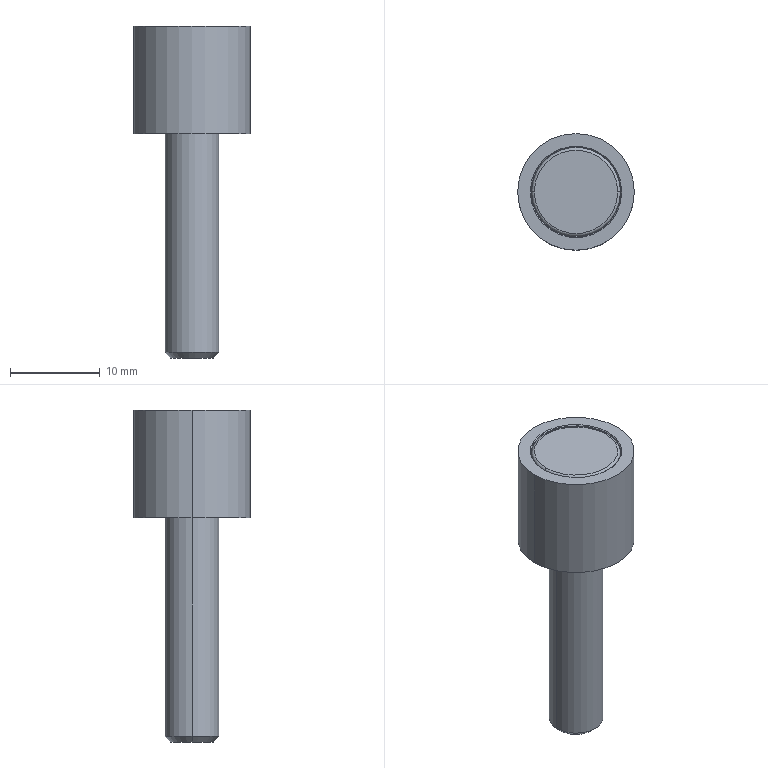Part | NX | features BREP 1 | 1 solid | 19 faces | box 13 x 13 x 37 mm | volume 2288 mm3 | cylinder 8 | plane 5 | cone 4 | torus 2 | commonest cylinder face diameters 6 x2 9.9 x2 10 x2 13 x2
STEP:
#1=CARTESIAN_POINT('',(4.65,0.,29.));
#2=VERTEX_POINT('',#1);
#3=CARTESIAN_POINT('',(-4.65,0.,29.));
#4=VERTEX_POINT('',#3);
#5=CARTESIAN_POINT('',(0.,0.,29.));
#6=DIRECTION('',(0.,0.,1.));
#7=DIRECTION('',(1.,0.,0.));
#8=AXIS2_PLACEMENT_3D('',#5,#6,#7);
#9=CIRCLE('',#8,4.65);
#10=EDGE_CURVE('',#2,#4,#9,.T.);
#11=ORIENTED_EDGE('',*,*,#10,.T.);
#12=CARTESIAN_POINT('',(0.,0.,29.));
#13=DIRECTION('',(0.,0.,1.));
#14=DIRECTION('',(1.,0.,0.));
#15=AXIS2_PLACEMENT_3D('',#12,#13,#14);
#16=CIRCLE('',#15,4.65);
#17=EDGE_CURVE('',#4,#2,#16,.T.);
#18=ORIENTED_EDGE('',*,*,#17,.T.);
#19=EDGE_LOOP('',(#11,#18));
#20=FACE_BOUND('',#19,.T.);
#21=CARTESIAN_POINT('',(4.65,0.,29.));
#22=DIRECTION('',(0.,0.,-1.));
#23=DIRECTION('',(-1.,0.,0.));
#24=AXIS2_PLACEMENT_3D('',#21,#22,#23);
#25=PLANE('',#24);
#26=ADVANCED_FACE('',(#20),#25,.F.);
#27=CARTESIAN_POINT('',(-4.95,0.,28.7));
#28=VERTEX_POINT('',#27);
#29=CARTESIAN_POINT('',(-4.65,0.,28.7));
#30=DIRECTION('',(0.,1.,0.));
#31=DIRECTION('',(-1.,0.,0.));
#32=AXIS2_PLACEMENT_3D('',#29,#30,#31);
#33=CIRCLE('',#32,0.3);
#34=EDGE_CURVE('',#4,#28,#33,.F.);
#35=ORIENTED_EDGE('',*,*,#34,.T.);
#36=CARTESIAN_POINT('',(4.95,0.,28.7));
#37=VERTEX_POINT('',#36);
#38=CARTESIAN_POINT('',(0.,0.,28.7));
#39=DIRECTION('',(0.,0.,1.));
#40=DIRECTION('',(1.,0.,0.));
#41=AXIS2_PLACEMENT_3D('',#38,#39,#40);
#42=CIRCLE('',#41,4.95);
#43=EDGE_CURVE('',#28,#37,#42,.T.);
#44=ORIENTED_EDGE('',*,*,#43,.T.);
#45=CARTESIAN_POINT('',(4.65,0.,28.7));
#46=DIRECTION('',(0.,-1.,0.));
#47=DIRECTION('',(0.,0.,-1.));
#48=AXIS2_PLACEMENT_3D('',#45,#46,#47);
#49=CIRCLE('',#48,0.3);
#50=EDGE_CURVE('',#2,#37,#49,.F.);
#51=ORIENTED_EDGE('',*,*,#50,.F.);
#52=ORIENTED_EDGE('',*,*,#17,.F.);
#53=EDGE_LOOP('',(#35,#44,#51,#52));
#54=FACE_BOUND('',#53,.T.);
#55=CARTESIAN_POINT('',(0.,0.,28.7));
#56=DIRECTION('',(0.,0.,1.));
#57=DIRECTION('',(1.,0.,0.));
#58=AXIS2_PLACEMENT_3D('',#55,#56,#57);
#59=TOROIDAL_SURFACE('',#58,4.65,0.3);
#60=ADVANCED_FACE('',(#54),#59,.T.);
#61=CARTESIAN_POINT('',(-4.95,0.,24.));
#62=VERTEX_POINT('',#61);
#63=CARTESIAN_POINT('',(-4.95,0.,50.));
#64=DIRECTION('',(0.,0.,1.));
#65=VECTOR('',#64,1000.);
#66=LINE('',#63,#65);
#67=EDGE_CURVE('',#28,#62,#66,.F.);
#68=ORIENTED_EDGE('',*,*,#67,.T.);
#69=CARTESIAN_POINT('',(4.95,0.,24.));
#70=VERTEX_POINT('',#69);
#71=CARTESIAN_POINT('',(0.,0.,24.));
#72=DIRECTION('',(0.,0.,1.));
#73=DIRECTION('',(1.,0.,0.));
#74=AXIS2_PLACEMENT_3D('',#71,#72,#73);
#75=CIRCLE('',#74,4.95);
#76=EDGE_CURVE('',#62,#70,#75,.T.);
#77=ORIENTED_EDGE('',*,*,#76,.T.);
#78=CARTESIAN_POINT('',(4.95,0.,50.));
#79=DIRECTION('',(0.,0.,1.));
#80=VECTOR('',#79,1000.);
#81=LINE('',#78,#80);
#82=EDGE_CURVE('',#37,#70,#81,.F.);
#83=ORIENTED_EDGE('',*,*,#82,.F.);
#84=ORIENTED_EDGE('',*,*,#43,.F.);
#85=EDGE_LOOP('',(#68,#77,#83,#84));
#86=FACE_BOUND('',#85,.T.);
#87=CARTESIAN_POINT('',(0.,0.,50.));
#88=DIRECTION('',(0.,0.,1.));
#89=DIRECTION('',(1.,0.,0.));
#90=AXIS2_PLACEMENT_3D('',#87,#88,#89);
#91=CYLINDRICAL_SURFACE('',#90,4.95);
#92=ADVANCED_FACE('',(#86),#91,.T.);
#93=CARTESIAN_POINT('',(5.,0.,24.));
#94=VERTEX_POINT('',#93);
#95=CARTESIAN_POINT('',(-5.,0.,24.));
#96=VERTEX_POINT('',#95);
#97=CARTESIAN_POINT('',(0.,0.,24.));
#98=DIRECTION('',(0.,0.,1.));
#99=DIRECTION('',(1.,0.,0.));
#100=AXIS2_PLACEMENT_3D('',#97,#98,#99);
#101=CIRCLE('',#100,5.);
#102=EDGE_CURVE('',#94,#96,#101,.T.);
#103=ORIENTED_EDGE('',*,*,#102,.T.);
#104=CARTESIAN_POINT('',(0.,0.,24.));
#105=DIRECTION('',(0.,0.,1.));
#106=DIRECTION('',(1.,0.,0.));
#107=AXIS2_PLACEMENT_3D('',#104,#105,#106);
#108=CIRCLE('',#107,5.);
#109=EDGE_CURVE('',#96,#94,#108,.T.);
#110=ORIENTED_EDGE('',*,*,#109,.T.);
#111=EDGE_LOOP('',(#103,#110));
#112=FACE_BOUND('',#111,.T.);
#113=CARTESIAN_POINT('',(0.,0.,24.));
#114=DIRECTION('',(0.,0.,1.));
#115=DIRECTION('',(1.,0.,0.));
#116=AXIS2_PLACEMENT_3D('',#113,#114,#115);
#117=CIRCLE('',#116,4.95);
#118=EDGE_CURVE('',#70,#62,#117,.T.);
#119=ORIENTED_EDGE('',*,*,#118,.F.);
#120=ORIENTED_EDGE('',*,*,#76,.F.);
#121=EDGE_LOOP('',(#119,#120));
#122=FACE_BOUND('',#121,.T.);
#123=CARTESIAN_POINT('',(5.,0.,24.));
#124=DIRECTION('',(0.,0.,-1.));
#125=DIRECTION('',(-1.,0.,0.));
#126=AXIS2_PLACEMENT_3D('',#123,#124,#125);
#127=PLANE('',#126);
#128=ADVANCED_FACE('',(#112,#122),#127,.F.);
#129=CARTESIAN_POINT('',(-5.,0.,28.9));
#130=VERTEX_POINT('',#129);
#131=CARTESIAN_POINT('',(-5.,0.,50.));
#132=DIRECTION('',(0.,0.,1.));
#133=VECTOR('',#132,1000.);
#134=LINE('',#131,#133);
#135=EDGE_CURVE('',#130,#96,#134,.F.);
#136=ORIENTED_EDGE('',*,*,#135,.T.);
#137=ORIENTED_EDGE('',*,*,#102,.F.);
#138=CARTESIAN_POINT('',(5.,0.,28.9));
#139=VERTEX_POINT('',#138);
#140=CARTESIAN_POINT('',(5.,0.,50.));
#141=DIRECTION('',(0.,0.,1.));
#142=VECTOR('',#141,1000.);
#143=LINE('',#140,#142);
#144=EDGE_CURVE('',#139,#94,#143,.F.);
#145=ORIENTED_EDGE('',*,*,#144,.F.);
#146=CARTESIAN_POINT('',(0.,0.,28.9));
#147=DIRECTION('',(0.,0.,1.));
#148=DIRECTION('',(1.,0.,0.));
#149=AXIS2_PLACEMENT_3D('',#146,#147,#148);
#150=CIRCLE('',#149,5.);
#151=EDGE_CURVE('',#139,#130,#150,.T.);
#152=ORIENTED_EDGE('',*,*,#151,.T.);
#153=EDGE_LOOP('',(#136,#137,#145,#152));
#154=FACE_BOUND('',#153,.T.);
#155=CARTESIAN_POINT('',(0.,0.,50.));
#156=DIRECTION('',(0.,0.,1.));
#157=DIRECTION('',(1.,0.,0.));
#158=AXIS2_PLACEMENT_3D('',#155,#156,#157);
#159=CYLINDRICAL_SURFACE('',#158,5.);
#160=ADVANCED_FACE('',(#154),#159,.F.);
#161=CARTESIAN_POINT('',(-5.1,0.,29.));
#162=VERTEX_POINT('',#161);
#163=CARTESIAN_POINT('',(-5.1,0.,29.));
#164=DIRECTION('',(-0.7071,0.,0.7071));
#165=VECTOR('',#164,1000.);
#166=LINE('',#163,#165);
#167=EDGE_CURVE('',#162,#130,#166,.F.);
#168=ORIENTED_EDGE('',*,*,#167,.T.);
#169=ORIENTED_EDGE('',*,*,#151,.F.);
#170=CARTESIAN_POINT('',(5.1,0.,29.));
#171=VERTEX_POINT('',#170);
#172=CARTESIAN_POINT('',(5.1,0.,29.));
#173=DIRECTION('',(0.7071,0.,0.7071));
#174=VECTOR('',#173,1000.);
#175=LINE('',#172,#174);
#176=EDGE_CURVE('',#171,#139,#175,.F.);
#177=ORIENTED_EDGE('',*,*,#176,.F.);
#178=CARTESIAN_POINT('',(0.,0.,29.));
#179=DIRECTION('',(0.,0.,1.));
#180=DIRECTION('',(1.,0.,0.));
#181=AXIS2_PLACEMENT_3D('',#178,#179,#180);
#182=CIRCLE('',#181,5.1);
#183=EDGE_CURVE('',#171,#162,#182,.T.);
#184=ORIENTED_EDGE('',*,*,#183,.T.);
#185=EDGE_LOOP('',(#168,#169,#177,#184));
#186=FACE_BOUND('',#185,.T.);
#187=CARTESIAN_POINT('',(0.,0.,29.));
#188=DIRECTION('',(0.,0.,1.));
#189=DIRECTION('',(1.,0.,0.));
#190=AXIS2_PLACEMENT_3D('',#187,#188,#189);
#191=CONICAL_SURFACE('',#190,5.1,0.7854);
#192=ADVANCED_FACE('',(#186),#191,.F.);
#193=CARTESIAN_POINT('',(6.5,0.,29.));
#194=VERTEX_POINT('',#193);
#195=CARTESIAN_POINT('',(-6.5,0.,29.));
#196=VERTEX_POINT('',#195);
#197=CARTESIAN_POINT('',(0.,0.,29.));
#198=DIRECTION('',(0.,0.,1.));
#199=DIRECTION('',(1.,0.,0.));
#200=AXIS2_PLACEMENT_3D('',#197,#198,#199);
#201=CIRCLE('',#200,6.5);
#202=EDGE_CURVE('',#194,#196,#201,.T.);
#203=ORIENTED_EDGE('',*,*,#202,.T.);
#204=CARTESIAN_POINT('',(0.,0.,29.));
#205=DIRECTION('',(0.,0.,1.));
#206=DIRECTION('',(1.,0.,0.));
#207=AXIS2_PLACEMENT_3D('',#204,#205,#206);
#208=CIRCLE('',#207,6.5);
#209=EDGE_CURVE('',#196,#194,#208,.T.);
#210=ORIENTED_EDGE('',*,*,#209,.T.);
#211=EDGE_LOOP('',(#203,#210));
#212=FACE_BOUND('',#211,.T.);
#213=ORIENTED_EDGE('',*,*,#183,.F.);
#214=CARTESIAN_POINT('',(0.,0.,29.));
#215=DIRECTION('',(0.,0.,1.));
#216=DIRECTION('',(1.,0.,0.));
#217=AXIS2_PLACEMENT_3D('',#214,#215,#216);
#218=CIRCLE('',#217,5.1);
#219=EDGE_CURVE('',#162,#171,#218,.T.);
#220=ORIENTED_EDGE('',*,*,#219,.F.);
#221=EDGE_LOOP('',(#213,#220));
#222=FACE_BOUND('',#221,.T.);
#223=CARTESIAN_POINT('',(6.5,0.,29.));
#224=DIRECTION('',(0.,0.,-1.));
#225=DIRECTION('',(-1.,0.,0.));
#226=AXIS2_PLACEMENT_3D('',#223,#224,#225);
#227=PLANE('',#226);
#228=ADVANCED_FACE('',(#212,#222),#227,.F.);
#229=CARTESIAN_POINT('',(-6.5,0.,17.));
#230=VERTEX_POINT('',#229);
#231=CARTESIAN_POINT('',(-6.5,0.,50.));
#232=DIRECTION('',(0.,0.,1.));
#233=VECTOR('',#232,1000.);
#234=LINE('',#231,#233);
#235=EDGE_CURVE('',#196,#230,#234,.F.);
#236=ORIENTED_EDGE('',*,*,#235,.T.);
#237=CARTESIAN_POINT('',(6.5,0.,17.));
#238=VERTEX_POINT('',#237);
#239=CARTESIAN_POINT('',(0.,0.,17.));
#240=DIRECTION('',(0.,0.,1.));
#241=DIRECTION('',(1.,0.,0.));
#242=AXIS2_PLACEMENT_3D('',#239,#240,#241);
#243=CIRCLE('',#242,6.5);
#244=EDGE_CURVE('',#230,#238,#243,.T.);
#245=ORIENTED_EDGE('',*,*,#244,.T.);
#246=CARTESIAN_POINT('',(6.5,0.,50.));
#247=DIRECTION('',(0.,0.,1.));
#248=VECTOR('',#247,1000.);
#249=LINE('',#246,#248);
#250=EDGE_CURVE('',#194,#238,#249,.F.);
#251=ORIENTED_EDGE('',*,*,#250,.F.);
#252=ORIENTED_EDGE('',*,*,#209,.F.);
#253=EDGE_LOOP('',(#236,#245,#251,#252));
#254=FACE_BOUND('',#253,.T.);
#255=CARTESIAN_POINT('',(0.,0.,50.));
#256=DIRECTION('',(0.,0.,1.));
#257=DIRECTION('',(1.,0.,0.));
#258=AXIS2_PLACEMENT_3D('',#255,#256,#257);
#259=CYLINDRICAL_SURFACE('',#258,6.5);
#260=ADVANCED_FACE('',(#254),#259,.T.);
#261=CARTESIAN_POINT('',(3.,0.,17.));
#262=VERTEX_POINT('',#261);
#263=CARTESIAN_POINT('',(-3.,0.,17.));
#264=VERTEX_POINT('',#263);
#265=CARTESIAN_POINT('',(0.,0.,17.));
#266=DIRECTION('',(0.,0.,1.));
#267=DIRECTION('',(1.,0.,0.));
#268=AXIS2_PLACEMENT_3D('',#265,#266,#267);
#269=CIRCLE('',#268,3.);
#270=EDGE_CURVE('',#262,#264,#269,.T.);
#271=ORIENTED_EDGE('',*,*,#270,.T.);
#272=CARTESIAN_POINT('',(0.,0.,17.));
#273=DIRECTION('',(0.,0.,1.));
#274=DIRECTION('',(1.,0.,0.));
#275=AXIS2_PLACEMENT_3D('',#272,#273,#274);
#276=CIRCLE('',#275,3.);
#277=EDGE_CURVE('',#264,#262,#276,.T.);
#278=ORIENTED_EDGE('',*,*,#277,.T.);
#279=EDGE_LOOP('',(#271,#278));
#280=FACE_BOUND('',#279,.T.);
#281=CARTESIAN_POINT('',(0.,0.,17.));
#282=DIRECTION('',(0.,0.,1.));
#283=DIRECTION('',(1.,0.,0.));
#284=AXIS2_PLACEMENT_3D('',#281,#282,#283);
#285=CIRCLE('',#284,6.5);
#286=EDGE_CURVE('',#238,#230,#285,.T.);
#287=ORIENTED_EDGE('',*,*,#286,.F.);
#288=ORIENTED_EDGE('',*,*,#244,.F.);
#289=EDGE_LOOP('',(#287,#288));
#290=FACE_BOUND('',#289,.T.);
#291=CARTESIAN_POINT('',(3.,0.,17.));
#292=DIRECTION('',(0.,0.,1.));
#293=DIRECTION('',(1.,0.,0.));
#294=AXIS2_PLACEMENT_3D('',#291,#292,#293);
#295=PLANE('',#294);
#296=ADVANCED_FACE('',(#280,#290),#295,.F.);
#297=CARTESIAN_POINT('',(-3.,0.,-7.386));
#298=VERTEX_POINT('',#297);
#299=CARTESIAN_POINT('',(-3.,0.,50.));
#300=DIRECTION('',(0.,0.,1.));
#301=VECTOR('',#300,1000.);
#302=LINE('',#299,#301);
#303=EDGE_CURVE('',#264,#298,#302,.F.);
#304=ORIENTED_EDGE('',*,*,#303,.T.);
#305=CARTESIAN_POINT('',(3.,0.,-7.386));
#306=VERTEX_POINT('',#305);
#307=CARTESIAN_POINT('',(0.,0.,-7.386));
#308=DIRECTION('',(0.,0.,1.));
#309=DIRECTION('',(1.,0.,0.));
#310=AXIS2_PLACEMENT_3D('',#307,#308,#309);
#311=CIRCLE('',#310,3.);
#312=EDGE_CURVE('',#298,#306,#311,.T.);
#313=ORIENTED_EDGE('',*,*,#312,.T.);
#314=CARTESIAN_POINT('',(3.,0.,50.));
#315=DIRECTION('',(0.,0.,1.));
#316=VECTOR('',#315,1000.);
#317=LINE('',#314,#316);
#318=EDGE_CURVE('',#262,#306,#317,.F.);
#319=ORIENTED_EDGE('',*,*,#318,.F.);
#320=ORIENTED_EDGE('',*,*,#277,.F.);
#321=EDGE_LOOP('',(#304,#313,#319,#320));
#322=FACE_BOUND('',#321,.T.);
#323=CARTESIAN_POINT('',(0.,0.,50.));
#324=DIRECTION('',(0.,0.,1.));
#325=DIRECTION('',(1.,0.,0.));
#326=AXIS2_PLACEMENT_3D('',#323,#324,#325);
#327=CYLINDRICAL_SURFACE('',#326,3.);
#328=ADVANCED_FACE('',(#322),#327,.T.);
#329=CARTESIAN_POINT('',(-2.386,0.,-8.));
#330=VERTEX_POINT('',#329);
#331=CARTESIAN_POINT('',(-2.386,0.,-8.));
#332=DIRECTION('',(-0.7071,0.,0.7071));
#333=VECTOR('',#332,1000.);
#334=LINE('',#331,#333);
#335=EDGE_CURVE('',#298,#330,#334,.F.);
#336=ORIENTED_EDGE('',*,*,#335,.T.);
#337=CARTESIAN_POINT('',(2.386,0.,-8.));
#338=VERTEX_POINT('',#337);
#339=CARTESIAN_POINT('',(0.,0.,-8.));
#340=DIRECTION('',(0.,0.,1.));
#341=DIRECTION('',(1.,0.,0.));
#342=AXIS2_PLACEMENT_3D('',#339,#340,#341);
#343=CIRCLE('',#342,2.386);
#344=EDGE_CURVE('',#330,#338,#343,.T.);
#345=ORIENTED_EDGE('',*,*,#344,.T.);
#346=CARTESIAN_POINT('',(2.386,0.,-8.));
#347=DIRECTION('',(0.7071,0.,0.7071));
#348=VECTOR('',#347,1000.);
#349=LINE('',#346,#348);
#350=EDGE_CURVE('',#306,#338,#349,.F.);
#351=ORIENTED_EDGE('',*,*,#350,.F.);
#352=ORIENTED_EDGE('',*,*,#312,.F.);
#353=EDGE_LOOP('',(#336,#345,#351,#352));
#354=FACE_BOUND('',#353,.T.);
#355=CARTESIAN_POINT('',(0.,0.,-8.));
#356=DIRECTION('',(0.,0.,1.));
#357=DIRECTION('',(1.,0.,0.));
#358=AXIS2_PLACEMENT_3D('',#355,#356,#357);
#359=CONICAL_SURFACE('',#358,2.386,0.7854);
#360=ADVANCED_FACE('',(#354),#359,.T.);
#361=CARTESIAN_POINT('',(0.,0.,-8.));
#362=DIRECTION('',(0.,0.,1.));
#363=DIRECTION('',(1.,0.,0.));
#364=AXIS2_PLACEMENT_3D('',#361,#362,#363);
#365=CIRCLE('',#364,2.386);
#366=EDGE_CURVE('',#338,#330,#365,.T.);
#367=ORIENTED_EDGE('',*,*,#366,.F.);
#368=ORIENTED_EDGE('',*,*,#344,.F.);
#369=EDGE_LOOP('',(#367,#368));
#370=FACE_BOUND('',#369,.T.);
#371=CARTESIAN_POINT('',(0.,0.,-8.));
#372=DIRECTION('',(0.,0.,1.));
#373=DIRECTION('',(1.,0.,0.));
#374=AXIS2_PLACEMENT_3D('',#371,#372,#373);
#375=PLANE('',#374);
#376=ADVANCED_FACE('',(#370),#375,.F.);
#377=ORIENTED_EDGE('',*,*,#366,.T.);
#378=ORIENTED_EDGE('',*,*,#335,.F.);
#379=CARTESIAN_POINT('',(0.,0.,-7.386));
#380=DIRECTION('',(0.,0.,1.));
#381=DIRECTION('',(1.,0.,0.));
#382=AXIS2_PLACEMENT_3D('',#379,#380,#381);
#383=CIRCLE('',#382,3.);
#384=EDGE_CURVE('',#306,#298,#383,.T.);
#385=ORIENTED_EDGE('',*,*,#384,.F.);
#386=ORIENTED_EDGE('',*,*,#350,.T.);
#387=EDGE_LOOP('',(#377,#378,#385,#386));
#388=FACE_BOUND('',#387,.T.);
#389=CARTESIAN_POINT('',(0.,0.,-8.));
#390=DIRECTION('',(0.,0.,1.));
#391=DIRECTION('',(1.,0.,0.));
#392=AXIS2_PLACEMENT_3D('',#389,#390,#391);
#393=CONICAL_SURFACE('',#392,2.386,0.7854);
#394=ADVANCED_FACE('',(#388),#393,.T.);
#395=ORIENTED_EDGE('',*,*,#384,.T.);
#396=ORIENTED_EDGE('',*,*,#303,.F.);
#397=ORIENTED_EDGE('',*,*,#270,.F.);
#398=ORIENTED_EDGE('',*,*,#318,.T.);
#399=EDGE_LOOP('',(#395,#396,#397,#398));
#400=FACE_BOUND('',#399,.T.);
#401=CARTESIAN_POINT('',(0.,0.,50.));
#402=DIRECTION('',(0.,0.,1.));
#403=DIRECTION('',(1.,0.,0.));
#404=AXIS2_PLACEMENT_3D('',#401,#402,#403);
#405=CYLINDRICAL_SURFACE('',#404,3.);
#406=ADVANCED_FACE('',(#400),#405,.T.);
#407=ORIENTED_EDGE('',*,*,#286,.T.);
#408=ORIENTED_EDGE('',*,*,#235,.F.);
#409=ORIENTED_EDGE('',*,*,#202,.F.);
#410=ORIENTED_EDGE('',*,*,#250,.T.);
#411=EDGE_LOOP('',(#407,#408,#409,#410));
#412=FACE_BOUND('',#411,.T.);
#413=CARTESIAN_POINT('',(0.,0.,50.));
#414=DIRECTION('',(0.,0.,1.));
#415=DIRECTION('',(1.,0.,0.));
#416=AXIS2_PLACEMENT_3D('',#413,#414,#415);
#417=CYLINDRICAL_SURFACE('',#416,6.5);
#418=ADVANCED_FACE('',(#412),#417,.T.);
#419=CARTESIAN_POINT('',(0.,0.,28.9));
#420=DIRECTION('',(0.,0.,1.));
#421=DIRECTION('',(1.,0.,0.));
#422=AXIS2_PLACEMENT_3D('',#419,#420,#421);
#423=CIRCLE('',#422,5.);
#424=EDGE_CURVE('',#130,#139,#423,.T.);
#425=ORIENTED_EDGE('',*,*,#424,.F.);
#426=ORIENTED_EDGE('',*,*,#167,.F.);
#427=ORIENTED_EDGE('',*,*,#219,.T.);
#428=ORIENTED_EDGE('',*,*,#176,.T.);
#429=EDGE_LOOP('',(#425,#426,#427,#428));
#430=FACE_BOUND('',#429,.T.);
#431=CARTESIAN_POINT('',(0.,0.,29.));
#432=DIRECTION('',(0.,0.,1.));
#433=DIRECTION('',(1.,0.,0.));
#434=AXIS2_PLACEMENT_3D('',#431,#432,#433);
#435=CONICAL_SURFACE('',#434,5.1,0.7854);
#436=ADVANCED_FACE('',(#430),#435,.F.);
#437=ORIENTED_EDGE('',*,*,#109,.F.);
#438=ORIENTED_EDGE('',*,*,#135,.F.);
#439=ORIENTED_EDGE('',*,*,#424,.T.);
#440=ORIENTED_EDGE('',*,*,#144,.T.);
#441=EDGE_LOOP('',(#437,#438,#439,#440));
#442=FACE_BOUND('',#441,.T.);
#443=CARTESIAN_POINT('',(0.,0.,50.));
#444=DIRECTION('',(0.,0.,1.));
#445=DIRECTION('',(1.,0.,0.));
#446=AXIS2_PLACEMENT_3D('',#443,#444,#445);
#447=CYLINDRICAL_SURFACE('',#446,5.);
#448=ADVANCED_FACE('',(#442),#447,.F.);
#449=ORIENTED_EDGE('',*,*,#118,.T.);
#450=ORIENTED_EDGE('',*,*,#67,.F.);
#451=CARTESIAN_POINT('',(0.,0.,28.7));
#452=DIRECTION('',(0.,0.,1.));
#453=DIRECTION('',(1.,0.,0.));
#454=AXIS2_PLACEMENT_3D('',#451,#452,#453);
#455=CIRCLE('',#454,4.95);
#456=EDGE_CURVE('',#37,#28,#455,.T.);
#457=ORIENTED_EDGE('',*,*,#456,.F.);
#458=ORIENTED_EDGE('',*,*,#82,.T.);
#459=EDGE_LOOP('',(#449,#450,#457,#458));
#460=FACE_BOUND('',#459,.T.);
#461=CARTESIAN_POINT('',(0.,0.,50.));
#462=DIRECTION('',(0.,0.,1.));
#463=DIRECTION('',(1.,0.,0.));
#464=AXIS2_PLACEMENT_3D('',#461,#462,#463);
#465=CYLINDRICAL_SURFACE('',#464,4.95);
#466=ADVANCED_FACE('',(#460),#465,.T.);
#467=ORIENTED_EDGE('',*,*,#456,.T.);
#468=ORIENTED_EDGE('',*,*,#34,.F.);
#469=ORIENTED_EDGE('',*,*,#10,.F.);
#470=ORIENTED_EDGE('',*,*,#50,.T.);
#471=EDGE_LOOP('',(#467,#468,#469,#470));
#472=FACE_BOUND('',#471,.T.);
#473=CARTESIAN_POINT('',(0.,0.,28.7));
#474=DIRECTION('',(0.,0.,1.));
#475=DIRECTION('',(1.,0.,0.));
#476=AXIS2_PLACEMENT_3D('',#473,#474,#475);
#477=TOROIDAL_SURFACE('',#476,4.65,0.3);
#478=ADVANCED_FACE('',(#472),#477,.T.);
#479=CLOSED_SHELL('',(#26,#60,#92,#128,#160,#192,#228,#260,#296,#328,#360,#376,#394,#406,#418,#436,#448,#466,#478));
#480=MANIFOLD_SOLID_BREP('',#479);
#481=(LENGTH_UNIT()NAMED_UNIT(*)SI_UNIT(.MILLI.,.METRE.));
#482=UNCERTAINTY_MEASURE_WITH_UNIT(LENGTH_MEASURE(0.00001),#481,'','');
#483=(NAMED_UNIT(*)PLANE_ANGLE_UNIT()SI_UNIT($,.RADIAN.));
#484=(NAMED_UNIT(*)SI_UNIT($,.STERADIAN.)SOLID_ANGLE_UNIT());
#485=(GEOMETRIC_REPRESENTATION_CONTEXT(3)GLOBAL_UNCERTAINTY_ASSIGNED_CONTEXT((#482))GLOBAL_UNIT_ASSIGNED_CONTEXT((#481,#483,#484))REPRESENTATION_CONTEXT('',''));
#486=ADVANCED_BREP_SHAPE_REPRESENTATION('',(#480),#485);